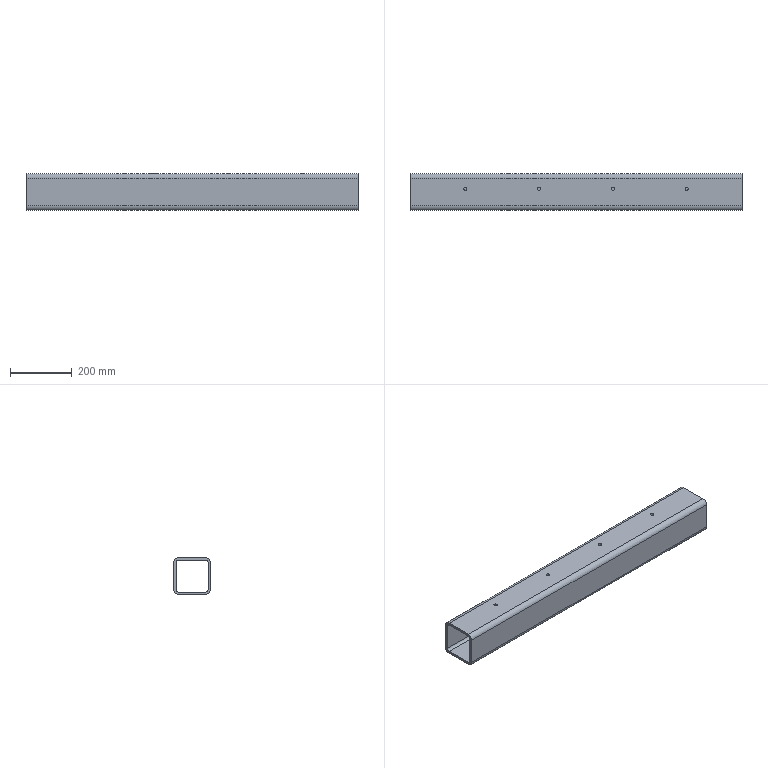Part | STEP file | Square tube 120X120X8-1079_Default<As machined> | 1 solid | 26 faces | box 1079 x 120 x 120 mm | volume 3686687 mm3 | cylinder 16 | plane 10 | commonest cylinder face diameters 10.2 x8 16 x4 32 x4